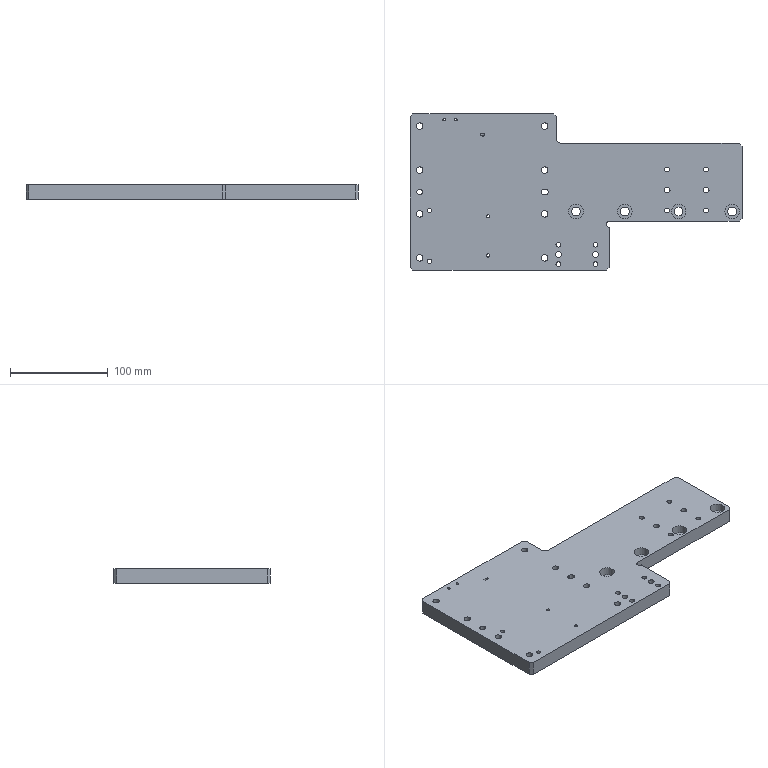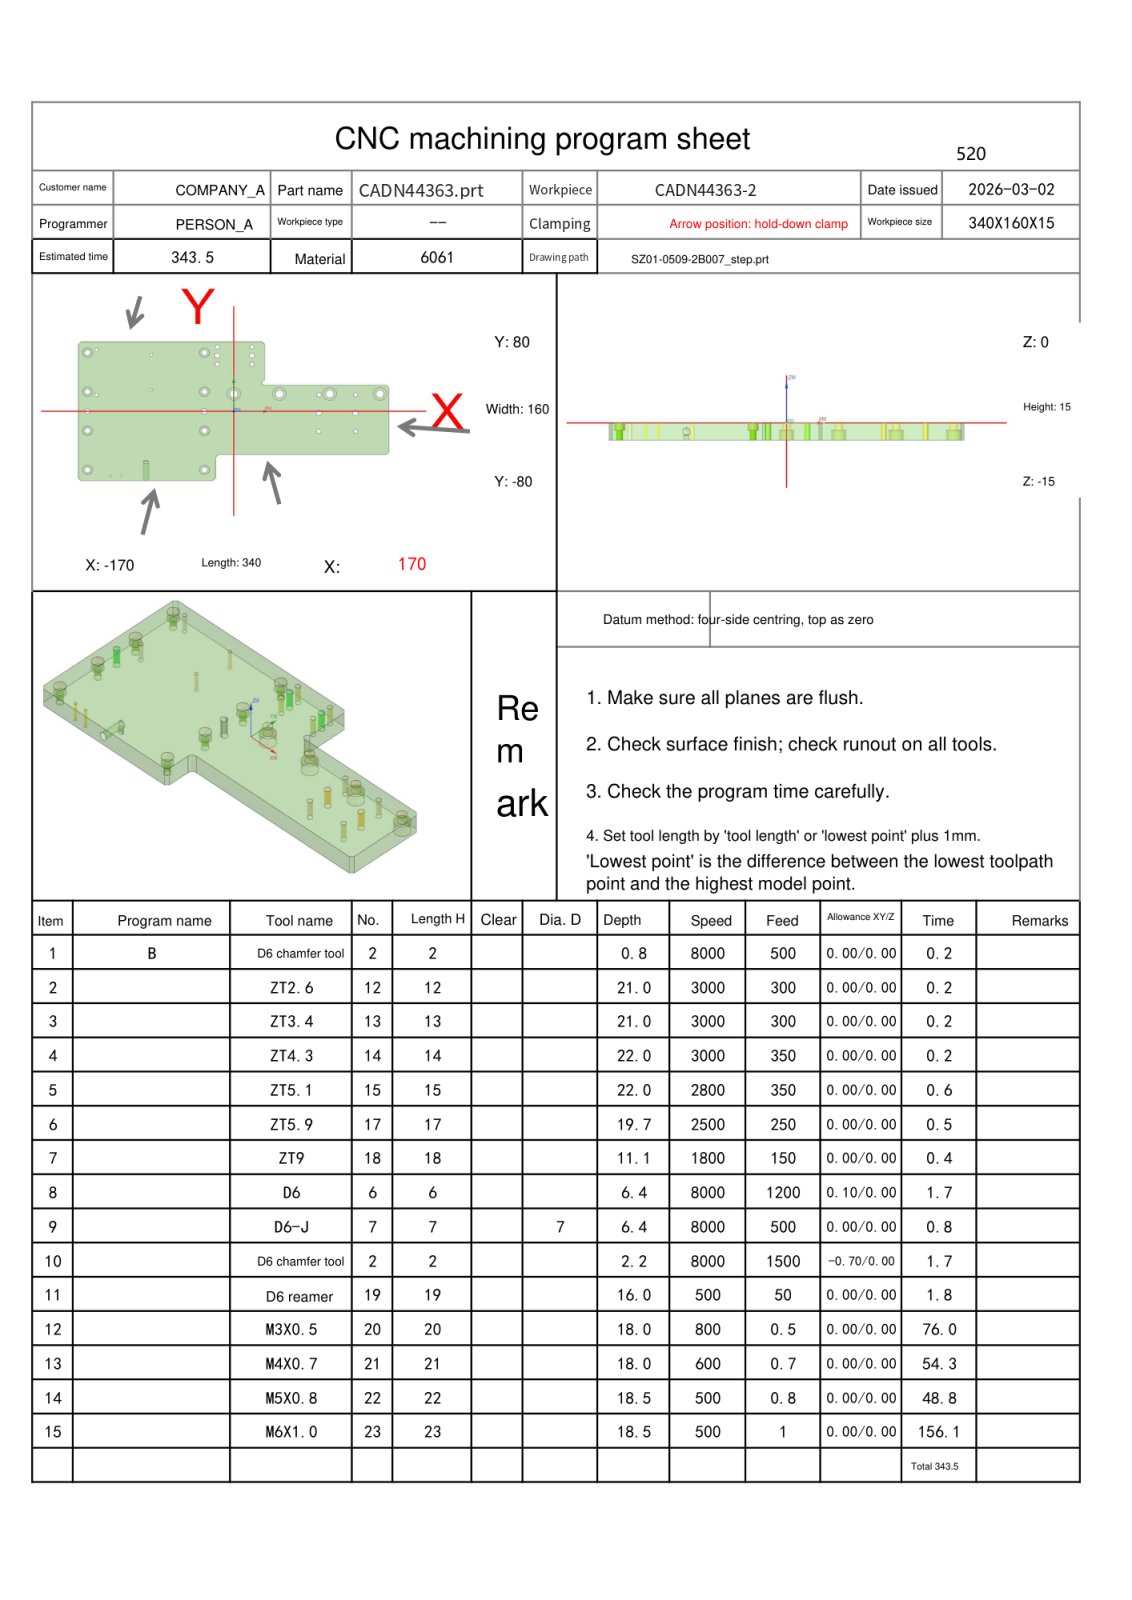NC program | NX | posted by the shop | part box 340 x 160 x 15 mm
Whole program:
%
O0001
(Machine time: 663.68 MIN)
(===Total Tool:14===)
(T2=D6 chamfer tool   D=6.   R=0.   D-  H02 Z=-2.2  )
(T12=ZT2.6  D=2.6  DR_a=118 D-  H12 Z=-21.  )
(T13=ZT3.4  D=3.4  DR_a=118 D-  H13 Z=-21.  )
(T14=ZT4.3  D=4.3  DR_a=118 D-  H14 Z=-22.  )
(T15=ZT5.1  D=5.1  DR_a=118 D-  H15 Z=-22.  )
(T17=ZT5.9  D=5.9  DR_a=120 D-  H17 Z=-19.7 )
(T18=ZT9    D=9.   DR_a=118 D-  H18 Z=-11.1 )
(T6=D6      D=6.   R=0.   D-  H06 Z=-6.4  )
(T7=D6-J    D=6.   R=0.   D7  H07 Z=-6.4  )
(T19=D6 reamer   D=6.   DR_a=180   D-  H19 Z=-16.  )
(T20=M3X0.5 D=2.5  DR_a=180 D-  H20 Z=-18.  )
(T21=M4X0.7 D=3.3  DR_a=180 D-  H21 Z=-18.  )
(T22=M5X0.8 D=4.2  DR_a=180 D-  H22 Z=-18.5 )
(T23=M6X1.0 D=5.   DR_a=180 D-  H23 Z=-18.5 )
G80 G90 G17 G49 G40
G91 G28 Z0
M01
N1 T02 M06
(D6 chamfer tool D=6. R=0. H=02 ce=0.00 di=0.00)
G00 G90 G54 X-90. Y25. M03 S8000
G43 H02 Z50.
M08
G98 G81 X-90. Y25. Z-.8 R1. F500.
Y65.
X-150. Y71.
X-160. Y67.5
Y22.5
X-150. Y19.
X-160. Y0.0
Y-22.5
Y-67.5
X-135. Y-74.
X-123.
X-32. Y-67.5
Y-22.5
Y22.5
X-18. Y54.
Y64.
X-32. Y67.5
X-18. Y74.
X20.
Y64.
Y54.
X0.0 Y20.
X50.
X93.275 Y19.
X105. Y20.
X93.275 Y-2.
Y-23.
X133.275
Y-2.
Y19.
X160. Y20.
G80
G00 Z50.
G91 G28 Z0.0
M05
M09
G91 G28 Z0.0
M01
N2 T12 M06
(ZT2.6 D=2.6 DR_a=118 H=12)
G00 G90 G54 X-135. Y-74. M03 S3000
G43 H12 Z50.
M08
G98 G83 X-135. Y-74. Z-21. R1. F300. Q2.
X-123.
G80
G00 Z50.
G91 G28 Z0.0
M05
M09
G91 G28 Z0.0
M01
N3 T13 M06
(ZT3.4 D=3.4 DR_a=118 H=13)
G00 G90 G54 X-90. Y65. M03 S3000
G43 H13 Z50.
M08
G98 G83 X-90. Y65. Z-21. R1. F300. Q2.
Y25.
G80
G00 Z50.
G91 G28 Z0.0
M05
M09
G91 G28 Z0.0
M01
N4 T14 M06
(ZT4.3 D=4.3 DR_a=118 H=14)
G00 G90 G54 X-150. Y71. M03 S3000
G43 H14 Z50.
M08
G98 G83 X-150. Y71. Z-22. R1. F350. Q3.
Y19.
G80
G00 Z50.
G91 G28 Z0.0
M05
M09
G91 G28 Z0.0
M01
N5 T15 M06
(ZT5.1 D=5.1 DR_a=118 H=15)
G00 G90 G54 X-18. Y54. M03 S2800
G43 H15 Z50.
M08
G98 G83 X-18. Y54. Z-22. R1. F350. Q3.
Y74.
X20.
Y54.
X93.275 Y19.
X133.275
Y-23.
X93.275
G80
G00 Z50.
G91 G28 Z0.0
M05
M09
G91 G28 Z0.0
M01
N6 T17 M06
(ZT5.9 D=5.9 DR_a=120 H=17)
G00 G90 G54 X-160. Y0.0 M03 S2500
G43 H17 Z50.
M08
G98 G83 X-160. Y0.0 Z-19.703 R1. F250. Q2.
X-18. Y64.
X20.
X93.275 Y-2.
X133.275
G80
G00 Z50.
G91 G28 Z0.0
M05
M09
G91 G28 Z0.0
M01
N7 T18 M06
(ZT9 D=9. DR_a=118 H=18)
G00 G90 G54 X0.0 Y20. M03 S1800
G43 H18 Z50.
M08
G98 G83 X0.0 Y20. Z-11.104 R1. F150. Q3.
X50.
X105.
X160.
G80
G00 Z50.
G91 G28 Z0.0
M05
M09
G91 G28 Z0.0
M01
N8 T06 M06
(D6  D=6. R=0. H=06 ce=0.10 di=0.00)
G00 G90 G54 X-160. Y22.5 M03 S8000
G43 H06 Z50.
M08
Z.5
G03 X-158.8 Y21.3 I1.2 J0.0 F1200.
X-157.6 Y22.5 I0.0 J1.2
X-157.6 Y22.5 Z0.0 I-2.4 J0.0
X-157.6 Y22.5 Z-.5 I-2.4 J0.0
X-157.6 Y22.5 Z-1. I-2.4 J0.0
X-157.6 Y22.5 Z-1.5 I-2.4 J0.0
X-157.6 Y22.5 Z-2. I-2.4 J0.0
X-157.6 Y22.5 Z-2.5 I-2.4 J0.0
X-157.6 Y22.5 Z-3. I-2.4 J0.0
X-157.6 Y22.5 Z-3.5 I-2.4 J0.0
X-157.6 Y22.5 Z-4. I-2.4 J0.0
X-157.6 Y22.5 Z-4.5 I-2.4 J0.0
X-157.6 Y22.5 Z-5. I-2.4 J0.0
X-157.6 Y22.5 Z-5.5 I-2.4 J0.0
X-157.6 Y22.5 Z-6. I-2.4 J0.0
X-159.258 Y20.217 Z-6.4 I-2.4 J0.0
X-157.6 Y22.5 I-.742 J2.283
X-160. Y24.9 I-2.4 J0.0
X-162.4 Y22.5 I0.0 J-2.4
X-160. Y20.1 I2.4 J0.0
X-159.258 Y20.217 I0.0 J2.4
X-158.429 Y21.359 I-.371 J1.141
X-159.629 Y22.559 I-1.2 J0.0
X-160. Y22.5 I0.0 J-1.2
G00 Z50.
Y67.5
Z.5
G03 X-158.8 Y66.3 I1.2 J0.0
X-157.6 Y67.5 I0.0 J1.2
X-157.6 Y67.5 Z0.0 I-2.4 J0.0
X-157.6 Y67.5 Z-.5 I-2.4 J0.0
X-157.6 Y67.5 Z-1. I-2.4 J0.0
X-157.6 Y67.5 Z-1.5 I-2.4 J0.0
X-157.6 Y67.5 Z-2. I-2.4 J0.0
X-157.6 Y67.5 Z-2.5 I-2.4 J0.0
X-157.6 Y67.5 Z-3. I-2.4 J0.0
X-157.6 Y67.5 Z-3.5 I-2.4 J0.0
X-157.6 Y67.5 Z-4. I-2.4 J0.0
X-157.6 Y67.5 Z-4.5 I-2.4 J0.0
X-157.6 Y67.5 Z-5. I-2.4 J0.0
X-157.6 Y67.5 Z-5.5 I-2.4 J0.0
X-157.6 Y67.5 Z-6. I-2.4 J0.0
X-159.258 Y65.217 Z-6.4 I-2.4 J0.0
X-157.6 Y67.5 I-.742 J2.283
X-160. Y69.9 I-2.4 J0.0
X-162.4 Y67.5 I0.0 J-2.4
X-160. Y65.1 I2.4 J0.0
X-159.258 Y65.217 I0.0 J2.4
X-158.429 Y66.359 I-.371 J1.141
X-159.629 Y67.559 I-1.2 J0.0
X-160. Y67.5 I0.0 J-1.2
G00 Z50.
Y-22.5
Z.5
G03 X-158.8 Y-23.7 I1.2 J0.0
X-157.6 Y-22.5 I0.0 J1.2
X-157.6 Y-22.5 Z0.0 I-2.4 J0.0
X-157.6 Y-22.5 Z-.5 I-2.4 J0.0
X-157.6 Y-22.5 Z-1. I-2.4 J0.0
X-157.6 Y-22.5 Z-1.5 I-2.4 J0.0
X-157.6 Y-22.5 Z-2. I-2.4 J0.0
X-157.6 Y-22.5 Z-2.5 I-2.4 J0.0
X-157.6 Y-22.5 Z-3. I-2.4 J0.0
X-157.6 Y-22.5 Z-3.5 I-2.4 J0.0
X-157.6 Y-22.5 Z-4. I-2.4 J0.0
X-157.6 Y-22.5 Z-4.5 I-2.4 J0.0
X-157.6 Y-22.5 Z-5. I-2.4 J0.0
X-157.6 Y-22.5 Z-5.5 I-2.4 J0.0
X-157.6 Y-22.5 Z-6. I-2.4 J0.0
X-159.258 Y-24.783 Z-6.4 I-2.4 J0.0
X-157.6 Y-22.5 I-.742 J2.283
X-160. Y-20.1 I-2.4 J0.0
X-162.4 Y-22.5 I0.0 J-2.4
X-160. Y-24.9 I2.4 J0.0
X-159.258 Y-24.783 I0.0 J2.4
X-158.429 Y-23.641 I-.371 J1.141
X-159.629 Y-22.441 I-1.2 J0.0
X-160. Y-22.5 I0.0 J-1.2
G00 Z50.
Y-67.5
Z.5
G03 X-158.8 Y-68.7 I1.2 J0.0
X-157.6 Y-67.5 I0.0 J1.2
X-157.6 Y-67.5 Z0.0 I-2.4 J0.0
X-157.6 Y-67.5 Z-.5 I-2.4 J0.0
X-157.6 Y-67.5 Z-1. I-2.4 J0.0
X-157.6 Y-67.5 Z-1.5 I-2.4 J0.0
X-157.6 Y-67.5 Z-2. I-2.4 J0.0
X-157.6 Y-67.5 Z-2.5 I-2.4 J0.0
X-157.6 Y-67.5 Z-3. I-2.4 J0.0
X-157.6 Y-67.5 Z-3.5 I-2.4 J0.0
X-157.6 Y-67.5 Z-4. I-2.4 J0.0
X-157.6 Y-67.5 Z-4.5 I-2.4 J0.0
X-157.6 Y-67.5 Z-5. I-2.4 J0.0
X-157.6 Y-67.5 Z-5.5 I-2.4 J0.0
X-157.6 Y-67.5 Z-6. I-2.4 J0.0
X-159.258 Y-69.783 Z-6.4 I-2.4 J0.0
X-157.6 Y-67.5 I-.742 J2.283
X-160. Y-65.1 I-2.4 J0.0
X-162.4 Y-67.5 I0.0 J-2.4
X-160. Y-69.9 I2.4 J0.0
X-159.258 Y-69.783 I0.0 J2.4
X-158.429 Y-68.641 I-.371 J1.141
X-159.629 Y-67.441 I-1.2 J0.0
X-160. Y-67.5 I0.0 J-1.2
G00 Z50.
X-32.
Z.5
G03 X-30.8 Y-68.7 I1.2 J0.0
X-29.6 Y-67.5 I0.0 J1.2
X-29.6 Y-67.5 Z0.0 I-2.4 J0.0
X-29.6 Y-67.5 Z-.5 I-2.4 J0.0
X-29.6 Y-67.5 Z-1. I-2.4 J0.0
X-29.6 Y-67.5 Z-1.5 I-2.4 J0.0
X-29.6 Y-67.5 Z-2. I-2.4 J0.0
X-29.6 Y-67.5 Z-2.5 I-2.4 J0.0
X-29.6 Y-67.5 Z-3. I-2.4 J0.0
X-29.6 Y-67.5 Z-3.5 I-2.4 J0.0
X-29.6 Y-67.5 Z-4. I-2.4 J0.0
X-29.6 Y-67.5 Z-4.5 I-2.4 J0.0
X-29.6 Y-67.5 Z-5. I-2.4 J0.0
X-29.6 Y-67.5 Z-5.5 I-2.4 J0.0
X-29.6 Y-67.5 Z-6. I-2.4 J0.0
X-31.258 Y-69.783 Z-6.4 I-2.4 J0.0
X-29.6 Y-67.5 I-.742 J2.283
X-32. Y-65.1 I-2.4 J0.0
X-34.4 Y-67.5 I0.0 J-2.4
X-32. Y-69.9 I2.4 J0.0
X-31.258 Y-69.783 I0.0 J2.4
X-30.429 Y-68.641 I-.371 J1.141
X-31.629 Y-67.441 I-1.2 J0.0
X-32. Y-67.5 I0.0 J-1.2
G00 Z50.
Y-22.5
Z.5
G03 X-30.8 Y-23.7 I1.2 J0.0
X-29.6 Y-22.5 I0.0 J1.2
X-29.6 Y-22.5 Z0.0 I-2.4 J0.0
X-29.6 Y-22.5 Z-.5 I-2.4 J0.0
X-29.6 Y-22.5 Z-1. I-2.4 J0.0
X-29.6 Y-22.5 Z-1.5 I-2.4 J0.0
X-29.6 Y-22.5 Z-2. I-2.4 J0.0
X-29.6 Y-22.5 Z-2.5 I-2.4 J0.0
X-29.6 Y-22.5 Z-3. I-2.4 J0.0
X-29.6 Y-22.5 Z-3.5 I-2.4 J0.0
X-29.6 Y-22.5 Z-4. I-2.4 J0.0
X-29.6 Y-22.5 Z-4.5 I-2.4 J0.0
X-29.6 Y-22.5 Z-5. I-2.4 J0.0
X-29.6 Y-22.5 Z-5.5 I-2.4 J0.0
X-29.6 Y-22.5 Z-6. I-2.4 J0.0
X-31.258 Y-24.783 Z-6.4 I-2.4 J0.0
X-29.6 Y-22.5 I-.742 J2.283
X-32. Y-20.1 I-2.4 J0.0
X-34.4 Y-22.5 I0.0 J-2.4
X-32. Y-24.9 I2.4 J0.0
X-31.258 Y-24.783 I0.0 J2.4
X-30.429 Y-23.641 I-.371 J1.141
X-31.629 Y-22.441 I-1.2 J0.0
X-32. Y-22.5 I0.0 J-1.2
G00 Z50.
Y22.5
Z.5
G03 X-30.8 Y21.3 I1.2 J0.0
X-29.6 Y22.5 I0.0 J1.2
X-29.6 Y22.5 Z0.0 I-2.4 J0.0
X-29.6 Y22.5 Z-.5 I-2.4 J0.0
X-29.6 Y22.5 Z-1. I-2.4 J0.0
X-29.6 Y22.5 Z-1.5 I-2.4 J0.0
X-29.6 Y22.5 Z-2. I-2.4 J0.0
X-29.6 Y22.5 Z-2.5 I-2.4 J0.0
X-29.6 Y22.5 Z-3. I-2.4 J0.0
X-29.6 Y22.5 Z-3.5 I-2.4 J0.0
X-29.6 Y22.5 Z-4. I-2.4 J0.0
X-29.6 Y22.5 Z-4.5 I-2.4 J0.0
X-29.6 Y22.5 Z-5. I-2.4 J0.0
X-29.6 Y22.5 Z-5.5 I-2.4 J0.0
X-29.6 Y22.5 Z-6. I-2.4 J0.0
X-31.258 Y20.217 Z-6.4 I-2.4 J0.0
X-29.6 Y22.5 I-.742 J2.283
X-32. Y24.9 I-2.4 J0.0
X-34.4 Y22.5 I0.0 J-2.4
X-32. Y20.1 I2.4 J0.0
X-31.258 Y20.217 I0.0 J2.4
X-30.429 Y21.359 I-.371 J1.141
X-31.629 Y22.559 I-1.2 J0.0
X-32. Y22.5 I0.0 J-1.2
G00 Z50.
Y67.5
Z.5
G03 X-30.8 Y66.3 I1.2 J0.0
X-29.6 Y67.5 I0.0 J1.2
X-29.6 Y67.5 Z0.0 I-2.4 J0.0
X-29.6 Y67.5 Z-.5 I-2.4 J0.0
X-29.6 Y67.5 Z-1. I-2.4 J0.0
X-29.6 Y67.5 Z-1.5 I-2.4 J0.0
X-29.6 Y67.5 Z-2. I-2.4 J0.0
X-29.6 Y67.5 Z-2.5 I-2.4 J0.0
X-29.6 Y67.5 Z-3. I-2.4 J0.0
X-29.6 Y67.5 Z-3.5 I-2.4 J0.0
X-29.6 Y67.5 Z-4. I-2.4 J0.0
X-29.6 Y67.5 Z-4.5 I-2.4 J0.0
X-29.6 Y67.5 Z-5. I-2.4 J0.0
X-29.6 Y67.5 Z-5.5 I-2.4 J0.0
X-29.6 Y67.5 Z-6. I-2.4 J0.0
X-31.258 Y65.217 Z-6.4 I-2.4 J0.0
X-29.6 Y67.5 I-.742 J2.283
X-32. Y69.9 I-2.4 J0.0
X-34.4 Y67.5 I0.0 J-2.4
X-32. Y65.1 I2.4 J0.0
X-31.258 Y65.217 I0.0 J2.4
X-30.429 Y66.359 I-.371 J1.141
X-31.629 Y67.559 I-1.2 J0.0
X-32. Y67.5 I0.0 J-1.2
G00 Z50.
G91 G28 Z0.0
M05
M09
G91 G28 Z0.0
M01
N9 T07 M06
(D6-J  D=6. R=0. H=07 ce=0.00 di=0.00)
G00 G90 G54 X-160. Y22.5 M03 S8000
G43 H07 Z50.
M08
Z0.0
G41 D07
G01 X-159.968 Y22.303 F500.
G03 X-158.742 Y21.258 I1.226 J.197
X-157.5 Y22.5 I0.0 J1.242
X-157.5 Y22.5 Z-5. I-2.5 J0.0
X-160.468 Y24.956 Z-6.4 I-2.5 J0.0
X-162.5 Y22.5 I.468 J-2.456
X-160. Y20. I2.5 J0.0
X-157.5 Y22.5 I0.0 J2.5
X-160. Y25. I-2.5 J0.0
X-160.468 Y24.956 I0.0 J-2.5
X-161.478 Y23.736 I.233 J-1.22
X-160.236 Y22.494 I1.242 J0.0
G01 X-160.2
G40 X-160. Y22.5
G00 Z50.
Y67.5
Z0.0
G41 D07
G01 X-159.968 Y67.303
G03 X-158.742 Y66.258 I1.226 J.197
X-157.5 Y67.5 I0.0 J1.242
X-157.5 Y67.5 Z-5. I-2.5 J0.0
X-160.468 Y69.956 Z-6.4 I-2.5 J0.0
X-162.5 Y67.5 I.468 J-2.456
X-160. Y65. I2.5 J0.0
X-157.5 Y67.5 I0.0 J2.5
X-160. Y70. I-2.5 J0.0
X-160.468 Y69.956 I0.0 J-2.5
X-161.478 Y68.736 I.233 J-1.22
X-160.236 Y67.494 I1.242 J0.0
G01 X-160.2
G40 X-160. Y67.5
G00 Z50.
Y-22.5
Z0.0
G41 D07
G01 X-159.968 Y-22.697
G03 X-158.742 Y-23.742 I1.226 J.197
X-157.5 Y-22.5 I0.0 J1.242
X-157.5 Y-22.5 Z-5. I-2.5 J0.0
X-160.468 Y-20.044 Z-6.4 I-2.5 J0.0
X-162.5 Y-22.5 I.468 J-2.456
X-160. Y-25. I2.5 J0.0
X-157.5 Y-22.5 I0.0 J2.5
X-160. Y-20. I-2.5 J0.0
X-160.468 Y-20.044 I0.0 J-2.5
X-161.478 Y-21.264 I.233 J-1.22
X-160.236 Y-22.506 I1.242 J0.0
G01 X-160.2
G40 X-160. Y-22.5
G00 Z50.
Y-67.5
Z0.0
G41 D07
G01 X-159.968 Y-67.697
G03 X-158.742 Y-68.742 I1.226 J.197
X-157.5 Y-67.5 I0.0 J1.242
X-157.5 Y-67.5 Z-5. I-2.5 J0.0
X-160.468 Y-65.044 Z-6.4 I-2.5 J0.0
X-162.5 Y-67.5 I.468 J-2.456
X-160. Y-70. I2.5 J0.0
X-157.5 Y-67.5 I0.0 J2.5
X-160. Y-65. I-2.5 J0.0
X-160.468 Y-65.044 I0.0 J-2.5
X-161.478 Y-66.264 I.233 J-1.22
X-160.236 Y-67.506 I1.242 J0.0
G01 X-160.2
G40 X-160. Y-67.5
G00 Z50.
X-32.
Z0.0
G41 D07
G01 X-31.968 Y-67.697
G03 X-30.742 Y-68.742 I1.226 J.197
X-29.5 Y-67.5 I0.0 J1.242
X-29.5 Y-67.5 Z-5. I-2.5 J0.0
X-32.468 Y-65.044 Z-6.4 I-2.5 J0.0
X-34.5 Y-67.5 I.468 J-2.456
X-32. Y-70. I2.5 J0.0
X-29.5 Y-67.5 I0.0 J2.5
X-32. Y-65. I-2.5 J0.0
X-32.468 Y-65.044 I0.0 J-2.5
X-33.478 Y-66.264 I.233 J-1.22
X-32.236 Y-67.506 I1.242 J0.0
G01 X-32.2
G40 X-32. Y-67.5
G00 Z50.
Y-22.5
Z0.0
G41 D07
G01 X-31.968 Y-22.697
G03 X-30.742 Y-23.742 I1.226 J.197
X-29.5 Y-22.5 I0.0 J1.242
X-29.5 Y-22.5 Z-5. I-2.5 J0.0
X-32.468 Y-20.044 Z-6.4 I-2.5 J0.0
X-34.5 Y-22.5 I.468 J-2.456
X-32. Y-25. I2.5 J0.0
X-29.5 Y-22.5 I0.0 J2.5
X-32. Y-20. I-2.5 J0.0
X-32.468 Y-20.044 I0.0 J-2.5
X-33.478 Y-21.264 I.233 J-1.22
X-32.236 Y-22.506 I1.242 J0.0
G01 X-32.2
G40 X-32. Y-22.5
G00 Z50.
Y22.5
Z0.0
G41 D07
G01 X-31.968 Y22.303
G03 X-30.742 Y21.258 I1.226 J.197
X-29.5 Y22.5 I0.0 J1.242
X-29.5 Y22.5 Z-5. I-2.5 J0.0
X-32.468 Y24.956 Z-6.4 I-2.5 J0.0
X-34.5 Y22.5 I.468 J-2.456
X-32. Y20. I2.5 J0.0
X-29.5 Y22.5 I0.0 J2.5
X-32. Y25. I-2.5 J0.0
X-32.468 Y24.956 I0.0 J-2.5
X-33.478 Y23.736 I.233 J-1.22
X-32.236 Y22.494 I1.242 J0.0
G01 X-32.2
G40 X-32. Y22.5
G00 Z50.
Y67.5
Z0.0
G41 D07
G01 X-31.968 Y67.303
G03 X-30.742 Y66.258 I1.226 J.197
X-29.5 Y67.5 I0.0 J1.242
X-29.5 Y67.5 Z-5. I-2.5 J0.0
X-32.468 Y69.956 Z-6.4 I-2.5 J0.0
X-34.5 Y67.5 I.468 J-2.456
X-32. Y65. I2.5 J0.0
X-29.5 Y67.5 I0.0 J2.5
X-32. Y70. I-2.5 J0.0
X-32.468 Y69.956 I0.0 J-2.5
X-33.478 Y68.736 I.233 J-1.22
X-32.236 Y67.494 I1.242 J0.0
G01 X-32.2
G40 X-32. Y67.5
G00 Z50.
G91 G28 Z0.0
M05
M09
G91 G28 Z0.0
M01
N10 T02 M06
(D6 chamfer tool D=6. R=0. H=02 ce=0.00 di=0.00)
G00 G90 G54 X-135. Y-74. M03 S8000
G43 H02 Z50.
M08
G98 G81 X-135. Y-74. Z-1.75 R3. F500.
X-123.
G80
G00 Z50.
G00 G90 X-90. Y65. M03 S8000
Z50.
G98 G81 X-90. Y65. Z-2.2 R3. F500.
Y25.
G80
G00 Z50.
G00 G90 X-149.907 Y70.306 M03 S8000
Z50.
Z-.5
G01 Z-1. F500.
X-149.8 Y69.5
G03 X-148.3 Y71. I0.0 J1.5
X-150. Y72.7 I-1.7 J0.0
X-151.7 Y71. I0.0 J-1.7
X-150. Y69.3 I1.7 J0.0
X-148.3 Y71. I0.0 J1.7
X-149.8 Y72.5 I-1.5 J0.0
G01 X-149.907 Y71.694
Z-.5
G00 Z50.
Y18.306
Z-.5
G01 Z-1.
X-149.8 Y17.5
G03 X-148.3 Y19. I0.0 J1.5
X-150. Y20.7 I-1.7 J0.0
X-151.7 Y19. I0.0 J-1.7
X-150. Y17.3 I1.7 J0.0
X-148.3 Y19. I0.0 J1.7
X-149.8 Y20.5 I-1.5 J0.0
G01 X-149.907 Y19.694
Z-.5
G00 Z50.
G00 G90 X92.866 Y-21.979 M03 S8000
Z50.
Z-.6
G01 Z-1.1 F500.
X92.675 Y-21.5
G03 X91.175 Y-23. I0.0 J-1.5
X93.275 Y-25.1 I2.1 J0.0
X95.375 Y-23. I0.0 J2.1
X93.275 Y-20.9 I-2.1 J0.0
X91.175 Y-23. I0.0 J-2.1
X92.675 Y-24.5 I1.5 J0.0
G01 X92.866 Y-24.021
Z-.6
G00 Z50.
X132.866 Y-21.979
Z-.6
G01 Z-1.1
X132.675 Y-21.5
G03 X131.175 Y-23. I0.0 J-1.5
X133.275 Y-25.1 I2.1 J0.0
X135.375 Y-23. I0.0 J2.1
X133.275 Y-20.9 I-2.1 J0.0
X131.175 Y-23. I0.0 J-2.1
X132.675 Y-24.5 I1.5 J0.0
G01 X132.866 Y-24.021
Z-.6
G00 Z50.
Y20.021
Z-.6
G01 Z-1.1
X132.675 Y20.5
G03 X131.175 Y19. I0.0 J-1.5
X133.275 Y16.9 I2.1 J0.0
X135.375 Y19. I0.0 J2.1
X133.275 Y21.1 I-2.1 J0.0
X131.175 Y19. I0.0 J-2.1
X132.675 Y17.5 I1.5 J0.0
G01 X132.866 Y17.979
Z-.6
G00 Z50.
X92.866 Y20.021
Z-.6
G01 Z-1.1
X92.675 Y20.5
G03 X91.175 Y19. I0.0 J-1.5
X93.275 Y16.9 I2.1 J0.0
X95.375 Y19. I0.0 J2.1
X93.275 Y21.1 I-2.1 J0.0
X91.175 Y19. I0.0 J-2.1
X92.675 Y17.5 I1.5 J0.0
G01 X92.866 Y17.979
Z-.6
G00 Z50.
X20.409 Y52.979
Z-.6
G01 Z-1.1
X20.6 Y52.5
G03 X22.1 Y54. I0.0 J1.5
X20. Y56.1 I-2.1 J0.0
X17.9 Y54. I0.0 J-2.1
X20. Y51.9 I2.1 J0.0
X22.1 Y54. I0.0 J2.1
X20.6 Y55.5 I-1.5 J0.0
G01 X20.409 Y55.021
Z-.6
G00 Z50.
Y72.979
Z-.6
G01 Z-1.1
X20.6 Y72.5
G03 X22.1 Y74. I0.0 J1.5
X20. Y76.1 I-2.1 J0.0
X17.9 Y74. I0.0 J-2.1
X20. Y71.9 I2.1 J0.0
X22.1 Y74. I0.0 J2.1
X20.6 Y75.5 I-1.5 J0.0
G01 X20.409 Y75.021
Z-.6
G00 Z50.
X-17.591 Y72.979
Z-.6
G01 Z-1.1
X-17.4 Y72.5
G03 X-15.9 Y74. I0.0 J1.5
X-18. Y76.1 I-2.1 J0.0
X-20.1 Y74. I0.0 J-2.1
X-18. Y71.9 I2.1 J0.0
X-15.9 Y74. I0.0 J2.1
X-17.4 Y75.5 I-1.5 J0.0
G01 X-17.591 Y75.021
Z-.6
G00 Z50.
Y52.979
Z-.6
G01 Z-1.1
X-17.4 Y52.5
G03 X-15.9 Y54. I0.0 J1.5
X-18. Y56.1 I-2.1 J0.0
X-20.1 Y54. I0.0 J-2.1
X-18. Y51.9 I2.1 J0.0
X-15.9 Y54. I0.0 J2.1
X-17.4 Y55.5 I-1.5 J0.0
G01 X-17.591 Y55.021
Z-.6
G00 Z50.
G00 G90 X132.663 Y-.853 M03 S8000
Z50.
Z-.5
G01 Z-1. F500.
X132.475 Y-.5
G03 X130.975 Y-2. I0.0 J-1.5
X133.275 Y-4.3 I2.3 J0.0
X135.575 Y-2. I0.0 J2.3
X133.275 Y.3 I-2.3 J0.0
X130.975 Y-2. I0.0 J-2.3
X132.475 Y-3.5 I1.5 J0.0
G01 X132.663 Y-3.147
Z-.5
G00 Z50.
X92.663 Y-.853
Z-.5
G01 Z-1.
X92.475 Y-.5
G03 X90.975 Y-2. I0.0 J-1.5
X93.275 Y-4.3 I2.3 J0.0
X95.575 Y-2. I0.0 J2.3
X93.275 Y.3 I-2.3 J0.0
X90.975 Y-2. I0.0 J-2.3
X92.475 Y-3.5 I1.5 J0.0
G01 X92.663 Y-3.147
Z-.5
G00 Z50.
X20.612 Y62.853
Z-.5
G01 Z-1.
X20.8 Y62.5
G03 X22.3 Y64. I0.0 J1.5
X20. Y66.3 I-2.3 J0.0
X17.7 Y64. I0.0 J-2.3
X20. Y61.7 I2.3 J0.0
X22.3 Y64. I0.0 J2.3
X20.8 Y65.5 I-1.5 J0.0
G01 X20.612 Y65.147
Z-.5
G00 Z50.
X-17.388 Y62.853
Z-.5
G01 Z-1.
X-17.2 Y62.5
G03 X-15.7 Y64. I0.0 J1.5
X-18. Y66.3 I-2.3 J0.0
X-20.3 Y64. I0.0 J-2.3
X-18. Y61.7 I2.3 J0.0
X-15.7 Y64. I0.0 J2.3
X-17.2 Y65.5 I-1.5 J0.0
G01 X-17.388 Y65.147
Z-.5
G00 Z50.
X-159.388 Y-1.147
Z-.5
G01 Z-1.
X-159.2 Y-1.5
G03 X-157.7 Y0.0 I0.0 J1.5
X-160. Y2.3 I-2.3 J0.0
X-162.3 Y0.0 I0.0 J-2.3
X-160. Y-2.3 I2.3 J0.0
X-157.7 Y0.0 I0.0 J2.3
X-159.2 Y1.5 I-1.5 J0.0
G01 X-159.388 Y1.147
Z-.5
G00 Z50.
G00 G90 X159.279 Y22.705 M03 S8000
Z50.
Z-.5
G01 Z-1. F800.
X159.2 Y23.
G03 X156.2 Y20. I0.0 J-3.
X160. Y16.2 I3.8 J0.0
X163.8 Y20. I0.0 J3.8
X160. Y23.8 I-3.8 J0.0
X156.2 Y20. I0.0 J-3.8
X159.2 Y17. I3. J0.0
G01 X159.279 Y17.295
Z-.5
G00 Z50.
X104.279 Y22.705
Z-.5
G01 Z-1.
X104.2 Y23.
G03 X101.2 Y20. I0.0 J-3.
X105. Y16.2 I3.8 J0.0
X108.8 Y20. I0.0 J3.8
X105. Y23.8 I-3.8 J0.0
X101.2 Y20. I0.0 J-3.8
X104.2 Y17. I3. J0.0
G01 X104.279 Y17.295
Z-.5
G00 Z50.
X49.279 Y22.705
Z-.5
G01 Z-1.
X49.2 Y23.
G03 X46.2 Y20. I0.0 J-3.
X50. Y16.2 I3.8 J0.0
X53.8 Y20. I0.0 J3.8
X50. Y23.8 I-3.8 J0.0
X46.2 Y20. I0.0 J-3.8
X49.2 Y17. I3. J0.0
G01 X49.279 Y17.295
Z-.5
G00 Z50.
X-.721 Y22.705
Z-.5
G01 Z-1.
X-.8 Y23.
G03 X-3.8 Y20. I0.0 J-3.
X0.0 Y16.2 I3.8 J0.0
X3.8 Y20. I0.0 J3.8
X0.0 Y23.8 I-3.8 J0.0
X-3.8 Y20. I0.0 J-3.8
X-.8 Y17. I3. J0.0
G01 X-.721 Y17.295
Z-.5
G00 Z50.
G00 G90 X-157.991 Y-63.143 M03 S8000
Z50.
Z2.5
G01 X-158.166 Y-63.061 Z2.43 F800.
X-158.601 Y-62.905 Z2.261
X-159.05 Y-62.792 Z2.093
X-159.507 Y-62.722 Z1.925
X-159.969 Y-62.697 Z1.756
X-160.431 Y-62.716 Z1.588
X-160.89 Y-62.78 Z1.419
X-161.34 Y-62.888 Z1.251
X-161.777 Y-63.038 Z1.083
X-162.198 Y-63.23 Z.914
X-162.599 Y-63.461 Z.746
X-162.976 Y-63.73 Z.577
X-163.325 Y-64.034 Z.409
X-163.643 Y-64.37 Z.241
X-163.927 Y-64.735 Z.072
X-164.175 Y-65.125 Z-.096
X-164.384 Y-65.538 Z-.265
X-164.552 Y-65.969 Z-.433
X-164.679 Y-66.414 Z-.601
X-164.761 Y-66.869 Z-.77
X-164.8 Y-67.33 Z-.938
Y-67.5 Z-1.
G03 X-160. Y-72.3 I4.8 J0.0
X-155.2 Y-67.5 I0.0 J4.8
X-160. Y-62.7 I-4.8 J0.0
X-164.8 Y-67.5 I0.0 J-4.8
X-164.774 Y-67.999 I4.8 J0.0
G01 Z1.5
G00 Z50.
X-157.991 Y-18.143
Z2.5
G01 X-158.166 Y-18.061 Z2.43
X-158.601 Y-17.905 Z2.261
X-159.05 Y-17.792 Z2.093
X-159.507 Y-17.722 Z1.925
X-159.969 Y-17.697 Z1.756
X-160.431 Y-17.716 Z1.588
X-160.89 Y-17.78 Z1.419
X-161.34 Y-17.888 Z1.251
X-161.777 Y-18.038 Z1.083
X-162.198 Y-18.23 Z.914
X-162.599 Y-18.461 Z.746
X-162.976 Y-18.73 Z.577
X-163.325 Y-19.034 Z.409
X-163.643 Y-19.37 Z.241
X-163.927 Y-19.735 Z.072
X-164.175 Y-20.125 Z-.096
X-164.384 Y-20.538 Z-.265
X-164.552 Y-20.969 Z-.433
X-164.679 Y-21.414 Z-.601
X-164.761 Y-21.869 Z-.77
X-164.8 Y-22.33 Z-.938
Y-22.5 Z-1.
G03 X-160. Y-27.3 I4.8 J0.0
X-155.2 Y-22.5 I0.0 J4.8
X-160. Y-17.7 I-4.8 J0.0
X-164.8 Y-22.5 I0.0 J-4.8
X-164.774 Y-22.999 I4.8 J0.0
G01 Z1.5
G00 Z50.
X-157.991 Y26.857
Z2.5
G01 X-158.166 Y26.939 Z2.43
X-158.601 Y27.095 Z2.261
X-159.05 Y27.208 Z2.093
X-159.507 Y27.278 Z1.925
X-159.969 Y27.303 Z1.756
X-160.431 Y27.284 Z1.588
X-160.89 Y27.22 Z1.419
X-161.34 Y27.112 Z1.251
X-161.777 Y26.962 Z1.083
X-162.198 Y26.77 Z.914
X-162.599 Y26.539 Z.746
X-162.976 Y26.27 Z.577
X-163.325 Y25.966 Z.409
X-163.643 Y25.63 Z.241
X-163.927 Y25.265 Z.072
X-164.175 Y24.875 Z-.096
X-164.384 Y24.462 Z-.265
X-164.552 Y24.031 Z-.433
X-164.679 Y23.586 Z-.601
X-164.761 Y23.131 Z-.77
X-164.8 Y22.67 Z-.938
Y22.5 Z-1.
G03 X-160. Y17.7 I4.8 J0.0
X-155.2 Y22.5 I0.0 J4.8
X-160. Y27.3 I-4.8 J0.0
X-164.8 Y22.5 I0.0 J-4.8
X-164.774 Y22.001 I4.8 J0.0
G01 Z1.5
G00 Z50.
X-157.991 Y71.857
Z2.5
G01 X-158.166 Y71.939 Z2.43
X-158.601 Y72.095 Z2.261
X-159.05 Y72.208 Z2.093
X-159.507 Y72.278 Z1.925
X-159.969 Y72.303 Z1.756
X-160.431 Y72.284 Z1.588
X-160.89 Y72.22 Z1.419
X-161.34 Y72.112 Z1.251
X-161.777 Y71.962 Z1.083
X-162.198 Y71.77 Z.914
X-162.599 Y71.539 Z.746
X-162.976 Y71.27 Z.577
X-163.325 Y70.966 Z.409
X-163.643 Y70.63 Z.241
X-163.927 Y70.265 Z.072
X-164.175 Y69.875 Z-.096
X-164.384 Y69.462 Z-.265
X-164.552 Y69.031 Z-.433
X-164.679 Y68.586 Z-.601
X-164.761 Y68.131 Z-.77
X-164.8 Y67.67 Z-.938
Y67.5 Z-1.
G03 X-160. Y62.7 I4.8 J0.0
X-155.2 Y67.5 I0.0 J4.8
X-160. Y72.3 I-4.8 J0.0
X-164.8 Y67.5 I0.0 J-4.8
X-164.774 Y67.001 I4.8 J0.0
G01 Z1.5
G00 Z50.
X-29.991 Y71.857
Z2.5
G01 X-30.166 Y71.939 Z2.43
X-30.601 Y72.095 Z2.261
X-31.05 Y72.208 Z2.093
X-31.507 Y72.278 Z1.925
X-31.969 Y72.303 Z1.756
X-32.431 Y72.284 Z1.588
X-32.89 Y72.22 Z1.419
X-33.34 Y72.112 Z1.251
X-33.777 Y71.962 Z1.083
X-34.198 Y71.77 Z.914
X-34.599 Y71.539 Z.746
X-34.976 Y71.27 Z.577
X-35.325 Y70.966 Z.409
X-35.643 Y70.63 Z.241
X-35.927 Y70.265 Z.072
X-36.175 Y69.875 Z-.096
X-36.384 Y69.462 Z-.265
X-36.552 Y69.031 Z-.433
X-36.679 Y68.586 Z-.601
X-36.761 Y68.131 Z-.77
X-36.8 Y67.67 Z-.938
Y67.5 Z-1.
G03 X-32. Y62.7 I4.8 J0.0
X-27.2 Y67.5 I0.0 J4.8
X-32. Y72.3 I-4.8 J0.0
X-36.8 Y67.5 I0.0 J-4.8
X-36.774 Y67.001 I4.8 J0.0
G01 Z1.5
G00 Z50.
X-29.991 Y26.857
Z2.5
G01 X-30.166 Y26.939 Z2.43
X-30.601 Y27.095 Z2.261
X-31.05 Y27.208 Z2.093
X-31.507 Y27.278 Z1.925
X-31.969 Y27.303 Z1.756
X-32.431 Y27.284 Z1.588
X-32.89 Y27.22 Z1.419
X-33.34 Y27.112 Z1.251
X-33.777 Y26.962 Z1.083
X-34.198 Y26.77 Z.914
X-34.599 Y26.539 Z.746
X-34.976 Y26.27 Z.577
X-35.325 Y25.966 Z.409
X-35.643 Y25.63 Z.241
X-35.927 Y25.265 Z.072
X-36.175 Y24.875 Z-.096
X-36.384 Y24.462 Z-.265
X-36.552 Y24.031 Z-.433
X-36.679 Y23.586 Z-.601
X-36.761 Y23.131 Z-.77
X-36.8 Y22.67 Z-.938
Y22.5 Z-1.
G03 X-32. Y17.7 I4.8 J0.0
X-27.2 Y22.5 I0.0 J4.8
X-32. Y27.3 I-4.8 J0.0
X-36.8 Y22.5 I0.0 J-4.8
X-36.774 Y22.001 I4.8 J0.0
G01 Z1.5
G00 Z50.
X-29.991 Y-18.143
Z2.5
G01 X-30.166 Y-18.061 Z2.43
X-30.601 Y-17.905 Z2.261
X-31.05 Y-17.792 Z2.093
X-31.507 Y-17.722 Z1.925
X-31.969 Y-17.697 Z1.756
X-32.431 Y-17.716 Z1.588
X-32.89 Y-17.78 Z1.419
X-33.34 Y-17.888 Z1.251
X-33.777 Y-18.038 Z1.083
X-34.198 Y-18.23 Z.914
X-34.599 Y-18.461 Z.746
X-34.976 Y-18.73 Z.577
X-35.325 Y-19.034 Z.409
X-35.643 Y-19.37 Z.241
X-35.927 Y-19.735 Z.072
X-36.175 Y-20.125 Z-.096
X-36.384 Y-20.538 Z-.265
X-36.552 Y-20.969 Z-.433
X-36.679 Y-21.414 Z-.601
X-36.761 Y-21.869 Z-.77
X-36.8 Y-22.33 Z-.938
Y-22.5 Z-1.
G03 X-32. Y-27.3 I4.8 J0.0
X-27.2 Y-22.5 I0.0 J4.8
X-32. Y-17.7 I-4.8 J0.0
X-36.8 Y-22.5 I0.0 J-4.8
X-36.774 Y-22.999 I4.8 J0.0
G01 Z1.5
G00 Z50.
X-29.991 Y-63.143
Z2.5
G01 X-30.166 Y-63.061 Z2.43
X-30.601 Y-62.905 Z2.261
X-31.05 Y-62.792 Z2.093
X-31.507 Y-62.722 Z1.925
X-31.969 Y-62.697 Z1.756
X-32.431 Y-62.716 Z1.588
X-32.89 Y-62.78 Z1.419
X-33.34 Y-62.888 Z1.251
X-33.777 Y-63.038 Z1.083
X-34.198 Y-63.23 Z.914
X-34.599 Y-63.461 Z.746
X-34.976 Y-63.73 Z.577
X-35.325 Y-64.034 Z.409
X-35.643 Y-64.37 Z.241
X-35.927 Y-64.735 Z.072
X-36.175 Y-65.125 Z-.096
X-36.384 Y-65.538 Z-.265
X-36.552 Y-65.969 Z-.433
X-36.679 Y-66.414 Z-.601
X-36.761 Y-66.869 Z-.77
X-36.8 Y-67.33 Z-.938
Y-67.5 Z-1.
G03 X-32. Y-72.3 I4.8 J0.0
X-27.2 Y-67.5 I0.0 J4.8
X-32. Y-62.7 I-4.8 J0.0
X-36.8 Y-67.5 I0.0 J-4.8
X-36.774 Y-67.999 I4.8 J0.0
G01 Z1.5
G00 Z50.
G00 G90 X-30.196 Y1.896 M03 S7000
Z50.
Z2.5
G01 X-30.228 Y1.92 Z2.486 F1500.
X-30.495 Y2.072 Z2.374
X-30.78 Y2.187 Z2.262
X-31.077 Y2.264 Z2.15
X-31.382 Y2.3 Z2.038
X-32.618 Z1.589
X-32.923 Y2.264 Z1.477
X-33.22 Y2.187 Z1.365
X-33.505 Y2.072 Z1.253
X-33.772 Y1.92 Z1.141
X-34.016 Y1.733 Z1.03
X-34.233 Y1.516 Z.918
X-34.42 Y1.272 Z.806
X-34.572 Y1.005 Z.694
X-34.687 Y.72 Z.582
X-34.764 Y.423 Z.47
X-34.8 Y.118 Z.358
Y-.118 Z.273
X-34.764 Y-.423 Z.161
X-34.687 Y-.72 Z.049
X-34.572 Y-1.005 Z-.063
X-34.42 Y-1.272 Z-.174
X-34.233 Y-1.516 Z-.286
X-34.016 Y-1.733 Z-.398
X-33.772 Y-1.92 Z-.51
X-33.505 Y-2.072 Z-.622
X-33.22 Y-2.187 Z-.734
X-32.923 Y-2.264 Z-.845
X-32.618 Y-2.3 Z-.957
X-32.5 Z-1.
X-31.5
G03 X-29.2 Y0.0 I0.0 J2.3
X-31.5 Y2.3 I-2.3 J0.0
G01 X-32.5
G03 X-34.8 Y0.0 I0.0 J-2.3
X-32.5 Y-2.3 I2.3 J0.0
G01 X-32.
Z1.5
G00 Z50.
G91 G28 Z0.0
M05
M09
G91 G28 Z0.0
M01
N11 T19 M06
(D6 reamer D=6. DR_a=180 H=19)
G00 G90 G54 X-160. Y0.0 M03 S500
G43 H19 Z50.
M08
G98 G81 X-160. Y0.0 Z-16. R1. F50.
X-18. Y64.
X20.
X93.275 Y-2.
X133.275
G80
G00 Z50.
G91 G28 Z0.0
M05
M09
G91 G28 Z0.0
M01
N12 T20 M06
(M3X0.5 D=2.5 DR_a=180 H=20)
G00 G90 G54 X-135. Y-74. M03 S800
G43 H20 Z50.
M08
G95
G98 G84 X-135. Y-74. Z-18. R1. F.5 Q5.
X-123.
G80
G94
G00 Z50.
G91 G28 Z0.0
M05
M09
G91 G28 Z0.0
M01
N13 T21 M06
(M4X0.7 D=3.3 DR_a=180 H=21)
G00 G90 G54 X-90. Y65. M03 S600
G43 H21 Z50.
M08
G95
G98 G84 X-90. Y65. Z-18. R1. F.7 Q4.
Y25.
G80
G94
G00 Z50.
G91 G28 Z0.0
M05
M09
G91 G28 Z0.0
M01
N14 T22 M06
(M5X0.8 D=4.2 DR_a=180 H=22)
G00 G90 G54 X-150. Y71. M03 S500
G43 H22 Z50.
M08
G95
G98 G84 X-150. Y71. Z-18.5 R1. F.8 Q3.
Y19.
G80
G94
G00 Z50.
G91 G28 Z0.0
M05
M09
G91 G28 Z0.0
M01
N15 T23 M06
(M6X1.0 D=5. DR_a=180 H=23)
G00 G90 G54 X-18. Y54. M03 S500
G43 H23 Z50.
M08
G95
G98 G84 X-18. Y54. Z-18.5 R1. F1. Q3.
Y74.
X20.
Y54.
X93.275 Y19.
X133.275
Y-23.
X93.275
G80
G94
G00 Z50.
M05
M09
G91 G28 Z0.0
G91 G28 Y0.0
M30
%